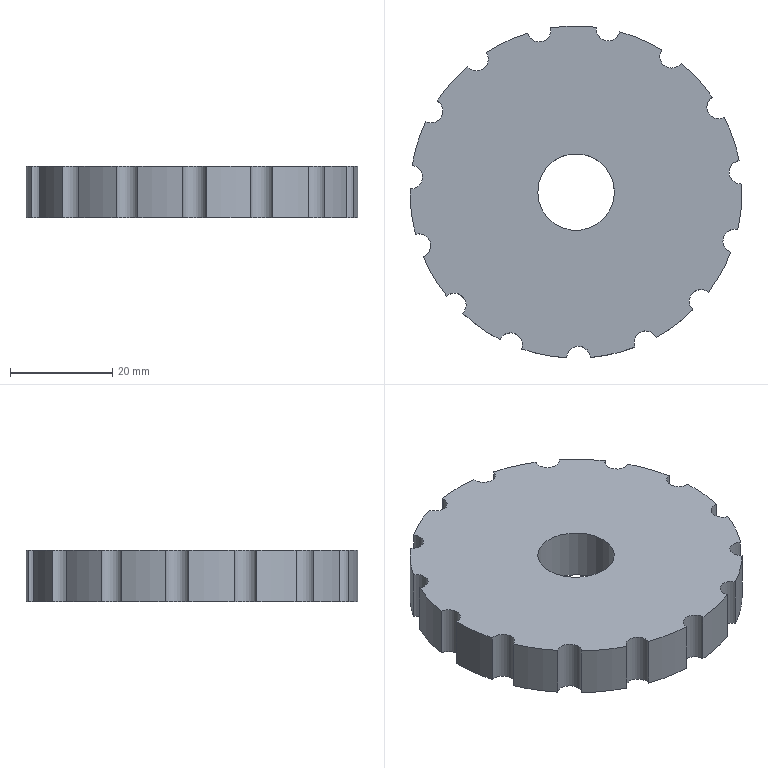Part | NX | features DATUM_CSYS 2, CYLINDER 1, EXTRUDE 1, SKETCH 1 | 1 solid | 33 faces | box 65 x 64.948 x 10 mm | volume 30179 mm3 | cylinder 31 | plane 2 | commonest cylinder face diameters 4.618 x15 65 x15 15 x1
STEP:
#1=CARTESIAN_POINT('',(16.782,27.832,0.));
#2=VERTEX_POINT('',#1);
#3=CARTESIAN_POINT('',(16.782,27.832,10.));
#4=VERTEX_POINT('',#3);
#5=CARTESIAN_POINT('',(16.782,27.832,0.));
#6=DIRECTION('',(0.,0.,1.));
#7=VECTOR('',#6,1000.);
#8=LINE('',#5,#7);
#9=EDGE_CURVE('',#2,#4,#8,.T.);
#10=ORIENTED_EDGE('',*,*,#9,.F.);
#11=CARTESIAN_POINT('',(8.539,31.358,0.));
#12=VERTEX_POINT('',#11);
#13=CARTESIAN_POINT('',(0.,0.,0.));
#14=DIRECTION('',(0.,0.,1.));
#15=DIRECTION('',(1.,0.,0.));
#16=AXIS2_PLACEMENT_3D('',#13,#14,#15);
#17=CIRCLE('',#16,32.5);
#18=EDGE_CURVE('',#2,#12,#17,.T.);
#19=ORIENTED_EDGE('',*,*,#18,.T.);
#20=CARTESIAN_POINT('',(8.539,31.358,10.));
#21=VERTEX_POINT('',#20);
#22=CARTESIAN_POINT('',(8.539,31.358,0.));
#23=DIRECTION('',(0.,0.,1.));
#24=VECTOR('',#23,1000.);
#25=LINE('',#22,#24);
#26=EDGE_CURVE('',#21,#12,#25,.F.);
#27=ORIENTED_EDGE('',*,*,#26,.F.);
#28=CARTESIAN_POINT('',(0.,0.,10.));
#29=DIRECTION('',(0.,0.,-1.));
#30=DIRECTION('',(1.,0.,0.));
#31=AXIS2_PLACEMENT_3D('',#28,#29,#30);
#32=CIRCLE('',#31,32.5);
#33=EDGE_CURVE('',#21,#4,#32,.T.);
#34=ORIENTED_EDGE('',*,*,#33,.T.);
#35=EDGE_LOOP('',(#10,#19,#27,#34));
#36=FACE_BOUND('',#35,.T.);
#37=CARTESIAN_POINT('',(0.,0.,0.));
#38=DIRECTION('',(0.,0.,1.));
#39=DIRECTION('',(1.,0.,0.));
#40=AXIS2_PLACEMENT_3D('',#37,#38,#39);
#41=CYLINDRICAL_SURFACE('',#40,32.5);
#42=ADVANCED_FACE('',(#36),#41,.T.);
#43=CARTESIAN_POINT('',(25.925,-19.599,0.));
#44=VERTEX_POINT('',#43);
#45=CARTESIAN_POINT('',(25.925,-19.599,10.));
#46=VERTEX_POINT('',#45);
#47=CARTESIAN_POINT('',(25.925,-19.599,0.));
#48=DIRECTION('',(0.,0.,1.));
#49=VECTOR('',#48,1000.);
#50=LINE('',#47,#49);
#51=EDGE_CURVE('',#44,#46,#50,.T.);
#52=ORIENTED_EDGE('',*,*,#51,.F.);
#53=CARTESIAN_POINT('',(30.294,-11.77,0.));
#54=VERTEX_POINT('',#53);
#55=CARTESIAN_POINT('',(0.,0.,0.));
#56=DIRECTION('',(0.,0.,1.));
#57=DIRECTION('',(1.,0.,0.));
#58=AXIS2_PLACEMENT_3D('',#55,#56,#57);
#59=CIRCLE('',#58,32.5);
#60=EDGE_CURVE('',#44,#54,#59,.T.);
#61=ORIENTED_EDGE('',*,*,#60,.T.);
#62=CARTESIAN_POINT('',(30.294,-11.77,10.));
#63=VERTEX_POINT('',#62);
#64=CARTESIAN_POINT('',(30.294,-11.77,0.));
#65=DIRECTION('',(0.,0.,1.));
#66=VECTOR('',#65,1000.);
#67=LINE('',#64,#66);
#68=EDGE_CURVE('',#63,#54,#67,.F.);
#69=ORIENTED_EDGE('',*,*,#68,.F.);
#70=CARTESIAN_POINT('',(0.,0.,10.));
#71=DIRECTION('',(0.,0.,-1.));
#72=DIRECTION('',(1.,0.,0.));
#73=AXIS2_PLACEMENT_3D('',#70,#71,#72);
#74=CIRCLE('',#73,32.5);
#75=EDGE_CURVE('',#63,#46,#74,.T.);
#76=ORIENTED_EDGE('',*,*,#75,.T.);
#77=EDGE_LOOP('',(#52,#61,#69,#76));
#78=FACE_BOUND('',#77,.T.);
#79=CARTESIAN_POINT('',(0.,0.,0.));
#80=DIRECTION('',(0.,0.,1.));
#81=DIRECTION('',(1.,0.,0.));
#82=AXIS2_PLACEMENT_3D('',#79,#80,#81);
#83=CYLINDRICAL_SURFACE('',#82,32.5);
#84=ADVANCED_FACE('',(#78),#83,.T.);
#85=CARTESIAN_POINT('',(20.555,25.174,10.));
#86=VERTEX_POINT('',#85);
#87=CARTESIAN_POINT('',(20.555,25.174,0.));
#88=VERTEX_POINT('',#87);
#89=CARTESIAN_POINT('',(20.555,25.174,0.));
#90=DIRECTION('',(0.,0.,1.));
#91=VECTOR('',#90,1000.);
#92=LINE('',#89,#91);
#93=EDGE_CURVE('',#86,#88,#92,.F.);
#94=ORIENTED_EDGE('',*,*,#93,.F.);
#95=CARTESIAN_POINT('',(26.651,18.6,10.));
#96=VERTEX_POINT('',#95);
#97=CARTESIAN_POINT('',(0.,0.,10.));
#98=DIRECTION('',(0.,0.,-1.));
#99=DIRECTION('',(1.,0.,0.));
#100=AXIS2_PLACEMENT_3D('',#97,#98,#99);
#101=CIRCLE('',#100,32.5);
#102=EDGE_CURVE('',#86,#96,#101,.T.);
#103=ORIENTED_EDGE('',*,*,#102,.T.);
#104=CARTESIAN_POINT('',(26.651,18.6,0.));
#105=VERTEX_POINT('',#104);
#106=CARTESIAN_POINT('',(26.651,18.6,0.));
#107=DIRECTION('',(0.,0.,1.));
#108=VECTOR('',#107,1000.);
#109=LINE('',#106,#108);
#110=EDGE_CURVE('',#105,#96,#109,.T.);
#111=ORIENTED_EDGE('',*,*,#110,.F.);
#112=CARTESIAN_POINT('',(0.,0.,0.));
#113=DIRECTION('',(0.,0.,1.));
#114=DIRECTION('',(1.,0.,0.));
#115=AXIS2_PLACEMENT_3D('',#112,#113,#114);
#116=CIRCLE('',#115,32.5);
#117=EDGE_CURVE('',#105,#88,#116,.T.);
#118=ORIENTED_EDGE('',*,*,#117,.T.);
#119=EDGE_LOOP('',(#94,#103,#111,#118));
#120=FACE_BOUND('',#119,.T.);
#121=CARTESIAN_POINT('',(0.,0.,0.));
#122=DIRECTION('',(0.,0.,1.));
#123=DIRECTION('',(1.,0.,0.));
#124=AXIS2_PLACEMENT_3D('',#121,#122,#123);
#125=CYLINDRICAL_SURFACE('',#124,32.5);
#126=ADVANCED_FACE('',(#120),#125,.T.);
#127=CARTESIAN_POINT('',(31.656,-7.36,0.));
#128=VERTEX_POINT('',#127);
#129=CARTESIAN_POINT('',(31.656,-7.36,10.));
#130=VERTEX_POINT('',#129);
#131=CARTESIAN_POINT('',(31.656,-7.36,0.));
#132=DIRECTION('',(0.,0.,1.));
#133=VECTOR('',#132,1000.);
#134=LINE('',#131,#133);
#135=EDGE_CURVE('',#128,#130,#134,.T.);
#136=ORIENTED_EDGE('',*,*,#135,.F.);
#137=CARTESIAN_POINT('',(32.462,1.569,0.));
#138=VERTEX_POINT('',#137);
#139=CARTESIAN_POINT('',(0.,0.,0.));
#140=DIRECTION('',(0.,0.,1.));
#141=DIRECTION('',(1.,0.,0.));
#142=AXIS2_PLACEMENT_3D('',#139,#140,#141);
#143=CIRCLE('',#142,32.5);
#144=EDGE_CURVE('',#128,#138,#143,.T.);
#145=ORIENTED_EDGE('',*,*,#144,.T.);
#146=CARTESIAN_POINT('',(32.462,1.569,10.));
#147=VERTEX_POINT('',#146);
#148=CARTESIAN_POINT('',(32.462,1.569,0.));
#149=DIRECTION('',(0.,0.,1.));
#150=VECTOR('',#149,1000.);
#151=LINE('',#148,#150);
#152=EDGE_CURVE('',#147,#138,#151,.F.);
#153=ORIENTED_EDGE('',*,*,#152,.F.);
#154=CARTESIAN_POINT('',(0.,0.,10.));
#155=DIRECTION('',(0.,0.,-1.));
#156=DIRECTION('',(1.,0.,0.));
#157=AXIS2_PLACEMENT_3D('',#154,#155,#156);
#158=CIRCLE('',#157,32.5);
#159=EDGE_CURVE('',#147,#130,#158,.T.);
#160=ORIENTED_EDGE('',*,*,#159,.T.);
#161=EDGE_LOOP('',(#136,#145,#153,#160));
#162=FACE_BOUND('',#161,.T.);
#163=CARTESIAN_POINT('',(0.,0.,0.));
#164=DIRECTION('',(0.,0.,1.));
#165=DIRECTION('',(1.,0.,0.));
#166=AXIS2_PLACEMENT_3D('',#163,#164,#165);
#167=CYLINDRICAL_SURFACE('',#166,32.5);
#168=ADVANCED_FACE('',(#162),#167,.T.);
#169=CARTESIAN_POINT('',(2.782,-32.381,0.));
#170=VERTEX_POINT('',#169);
#171=CARTESIAN_POINT('',(2.782,-32.381,10.));
#172=VERTEX_POINT('',#171);
#173=CARTESIAN_POINT('',(2.782,-32.381,0.));
#174=DIRECTION('',(0.,0.,1.));
#175=VECTOR('',#174,1000.);
#176=LINE('',#173,#175);
#177=EDGE_CURVE('',#170,#172,#176,.T.);
#178=ORIENTED_EDGE('',*,*,#177,.F.);
#179=CARTESIAN_POINT('',(11.524,-30.388,0.));
#180=VERTEX_POINT('',#179);
#181=CARTESIAN_POINT('',(0.,0.,0.));
#182=DIRECTION('',(0.,0.,1.));
#183=DIRECTION('',(1.,0.,0.));
#184=AXIS2_PLACEMENT_3D('',#181,#182,#183);
#185=CIRCLE('',#184,32.5);
#186=EDGE_CURVE('',#170,#180,#185,.T.);
#187=ORIENTED_EDGE('',*,*,#186,.T.);
#188=CARTESIAN_POINT('',(11.524,-30.388,10.));
#189=VERTEX_POINT('',#188);
#190=CARTESIAN_POINT('',(11.524,-30.388,0.));
#191=DIRECTION('',(0.,0.,1.));
#192=VECTOR('',#191,1000.);
#193=LINE('',#190,#192);
#194=EDGE_CURVE('',#189,#180,#193,.F.);
#195=ORIENTED_EDGE('',*,*,#194,.F.);
#196=CARTESIAN_POINT('',(0.,0.,10.));
#197=DIRECTION('',(0.,0.,-1.));
#198=DIRECTION('',(1.,0.,0.));
#199=AXIS2_PLACEMENT_3D('',#196,#197,#198);
#200=CIRCLE('',#199,32.5);
#201=EDGE_CURVE('',#189,#172,#200,.T.);
#202=ORIENTED_EDGE('',*,*,#201,.T.);
#203=EDGE_LOOP('',(#178,#187,#195,#202));
#204=FACE_BOUND('',#203,.T.);
#205=CARTESIAN_POINT('',(0.,0.,0.));
#206=DIRECTION('',(0.,0.,1.));
#207=DIRECTION('',(1.,0.,0.));
#208=AXIS2_PLACEMENT_3D('',#205,#206,#207);
#209=CYLINDRICAL_SURFACE('',#208,32.5);
#210=ADVANCED_FACE('',(#204),#209,.T.);
#211=CARTESIAN_POINT('',(4.011,32.252,0.));
#212=VERTEX_POINT('',#211);
#213=CARTESIAN_POINT('',(4.011,32.252,10.));
#214=VERTEX_POINT('',#213);
#215=CARTESIAN_POINT('',(4.011,32.252,0.));
#216=DIRECTION('',(0.,0.,1.));
#217=VECTOR('',#216,1000.);
#218=LINE('',#215,#217);
#219=EDGE_CURVE('',#212,#214,#218,.T.);
#220=ORIENTED_EDGE('',*,*,#219,.F.);
#221=CARTESIAN_POINT('',(-4.954,32.12,0.));
#222=VERTEX_POINT('',#221);
#223=CARTESIAN_POINT('',(0.,0.,0.));
#224=DIRECTION('',(0.,0.,1.));
#225=DIRECTION('',(1.,0.,0.));
#226=AXIS2_PLACEMENT_3D('',#223,#224,#225);
#227=CIRCLE('',#226,32.5);
#228=EDGE_CURVE('',#212,#222,#227,.T.);
#229=ORIENTED_EDGE('',*,*,#228,.T.);
#230=CARTESIAN_POINT('',(-4.954,32.12,10.));
#231=VERTEX_POINT('',#230);
#232=CARTESIAN_POINT('',(-4.954,32.12,0.));
#233=DIRECTION('',(0.,0.,1.));
#234=VECTOR('',#233,1000.);
#235=LINE('',#232,#234);
#236=EDGE_CURVE('',#231,#222,#235,.F.);
#237=ORIENTED_EDGE('',*,*,#236,.F.);
#238=CARTESIAN_POINT('',(0.,0.,10.));
#239=DIRECTION('',(0.,0.,-1.));
#240=DIRECTION('',(1.,0.,0.));
#241=AXIS2_PLACEMENT_3D('',#238,#239,#240);
#242=CIRCLE('',#241,32.5);
#243=EDGE_CURVE('',#231,#214,#242,.T.);
#244=ORIENTED_EDGE('',*,*,#243,.T.);
#245=EDGE_LOOP('',(#220,#229,#237,#244));
#246=FACE_BOUND('',#245,.T.);
#247=CARTESIAN_POINT('',(0.,0.,0.));
#248=DIRECTION('',(0.,0.,1.));
#249=DIRECTION('',(1.,0.,0.));
#250=AXIS2_PLACEMENT_3D('',#247,#248,#249);
#251=CYLINDRICAL_SURFACE('',#250,32.5);
#252=ADVANCED_FACE('',(#246),#251,.T.);
#253=CARTESIAN_POINT('',(22.888,-23.074,10.));
#254=VERTEX_POINT('',#253);
#255=CARTESIAN_POINT('',(22.888,-23.074,0.));
#256=VERTEX_POINT('',#255);
#257=CARTESIAN_POINT('',(22.888,-23.074,0.));
#258=DIRECTION('',(0.,0.,1.));
#259=VECTOR('',#258,1000.);
#260=LINE('',#257,#259);
#261=EDGE_CURVE('',#254,#256,#260,.F.);
#262=ORIENTED_EDGE('',*,*,#261,.F.);
#263=CARTESIAN_POINT('',(15.712,-28.45,10.));
#264=VERTEX_POINT('',#263);
#265=CARTESIAN_POINT('',(0.,0.,10.));
#266=DIRECTION('',(0.,0.,-1.));
#267=DIRECTION('',(1.,0.,0.));
#268=AXIS2_PLACEMENT_3D('',#265,#266,#267);
#269=CIRCLE('',#268,32.5);
#270=EDGE_CURVE('',#254,#264,#269,.T.);
#271=ORIENTED_EDGE('',*,*,#270,.T.);
#272=CARTESIAN_POINT('',(15.712,-28.45,0.));
#273=VERTEX_POINT('',#272);
#274=CARTESIAN_POINT('',(15.712,-28.45,0.));
#275=DIRECTION('',(0.,0.,1.));
#276=VECTOR('',#275,1000.);
#277=LINE('',#274,#276);
#278=EDGE_CURVE('',#273,#264,#277,.T.);
#279=ORIENTED_EDGE('',*,*,#278,.F.);
#280=CARTESIAN_POINT('',(0.,0.,0.));
#281=DIRECTION('',(0.,0.,1.));
#282=DIRECTION('',(1.,0.,0.));
#283=AXIS2_PLACEMENT_3D('',#280,#281,#282);
#284=CIRCLE('',#283,32.5);
#285=EDGE_CURVE('',#273,#256,#284,.T.);
#286=ORIENTED_EDGE('',*,*,#285,.T.);
#287=EDGE_LOOP('',(#262,#271,#279,#286));
#288=FACE_BOUND('',#287,.T.);
#289=CARTESIAN_POINT('',(0.,0.,0.));
#290=DIRECTION('',(0.,0.,1.));
#291=DIRECTION('',(1.,0.,0.));
#292=AXIS2_PLACEMENT_3D('',#289,#290,#291);
#293=CYLINDRICAL_SURFACE('',#292,32.5);
#294=ADVANCED_FACE('',(#288),#293,.T.);
#295=CARTESIAN_POINT('',(-29.434,13.781,0.));
#296=VERTEX_POINT('',#295);
#297=CARTESIAN_POINT('',(-29.434,13.781,10.));
#298=VERTEX_POINT('',#297);
#299=CARTESIAN_POINT('',(-29.434,13.781,0.));
#300=DIRECTION('',(0.,0.,1.));
#301=VECTOR('',#300,1000.);
#302=LINE('',#299,#301);
#303=EDGE_CURVE('',#296,#298,#302,.T.);
#304=ORIENTED_EDGE('',*,*,#303,.F.);
#305=CARTESIAN_POINT('',(-32.079,5.214,0.));
#306=VERTEX_POINT('',#305);
#307=CARTESIAN_POINT('',(0.,0.,0.));
#308=DIRECTION('',(0.,0.,1.));
#309=DIRECTION('',(1.,0.,0.));
#310=AXIS2_PLACEMENT_3D('',#307,#308,#309);
#311=CIRCLE('',#310,32.5);
#312=EDGE_CURVE('',#296,#306,#311,.T.);
#313=ORIENTED_EDGE('',*,*,#312,.T.);
#314=CARTESIAN_POINT('',(-32.079,5.214,10.));
#315=VERTEX_POINT('',#314);
#316=CARTESIAN_POINT('',(-32.079,5.214,0.));
#317=DIRECTION('',(0.,0.,1.));
#318=VECTOR('',#317,1000.);
#319=LINE('',#316,#318);
#320=EDGE_CURVE('',#315,#306,#319,.F.);
#321=ORIENTED_EDGE('',*,*,#320,.F.);
#322=CARTESIAN_POINT('',(0.,0.,10.));
#323=DIRECTION('',(0.,0.,-1.));
#324=DIRECTION('',(1.,0.,0.));
#325=AXIS2_PLACEMENT_3D('',#322,#323,#324);
#326=CIRCLE('',#325,32.5);
#327=EDGE_CURVE('',#315,#298,#326,.T.);
#328=ORIENTED_EDGE('',*,*,#327,.T.);
#329=EDGE_LOOP('',(#304,#313,#321,#328));
#330=FACE_BOUND('',#329,.T.);
#331=CARTESIAN_POINT('',(0.,0.,0.));
#332=DIRECTION('',(0.,0.,1.));
#333=DIRECTION('',(1.,0.,0.));
#334=AXIS2_PLACEMENT_3D('',#331,#332,#333);
#335=CYLINDRICAL_SURFACE('',#334,32.5);
#336=ADVANCED_FACE('',(#330),#335,.T.);
#337=CARTESIAN_POINT('',(-29.936,-12.652,0.));
#338=VERTEX_POINT('',#337);
#339=CARTESIAN_POINT('',(-29.936,-12.652,10.));
#340=VERTEX_POINT('',#339);
#341=CARTESIAN_POINT('',(-29.936,-12.652,0.));
#342=DIRECTION('',(0.,0.,1.));
#343=VECTOR('',#342,1000.);
#344=LINE('',#341,#343);
#345=EDGE_CURVE('',#338,#340,#344,.T.);
#346=ORIENTED_EDGE('',*,*,#345,.F.);
#347=CARTESIAN_POINT('',(-25.34,-20.35,0.));
#348=VERTEX_POINT('',#347);
#349=CARTESIAN_POINT('',(0.,0.,0.));
#350=DIRECTION('',(0.,0.,1.));
#351=DIRECTION('',(1.,0.,0.));
#352=AXIS2_PLACEMENT_3D('',#349,#350,#351);
#353=CIRCLE('',#352,32.5);
#354=EDGE_CURVE('',#338,#348,#353,.T.);
#355=ORIENTED_EDGE('',*,*,#354,.T.);
#356=CARTESIAN_POINT('',(-25.34,-20.35,10.));
#357=VERTEX_POINT('',#356);
#358=CARTESIAN_POINT('',(-25.34,-20.35,0.));
#359=DIRECTION('',(0.,0.,1.));
#360=VECTOR('',#359,1000.);
#361=LINE('',#358,#360);
#362=EDGE_CURVE('',#357,#348,#361,.F.);
#363=ORIENTED_EDGE('',*,*,#362,.F.);
#364=CARTESIAN_POINT('',(0.,0.,10.));
#365=DIRECTION('',(0.,0.,-1.));
#366=DIRECTION('',(1.,0.,0.));
#367=AXIS2_PLACEMENT_3D('',#364,#365,#366);
#368=CIRCLE('',#367,32.5);
#369=EDGE_CURVE('',#357,#340,#368,.T.);
#370=ORIENTED_EDGE('',*,*,#369,.T.);
#371=EDGE_LOOP('',(#346,#355,#363,#370));
#372=FACE_BOUND('',#371,.T.);
#373=CARTESIAN_POINT('',(0.,0.,0.));
#374=DIRECTION('',(0.,0.,1.));
#375=DIRECTION('',(1.,0.,0.));
#376=AXIS2_PLACEMENT_3D('',#373,#374,#375);
#377=CYLINDRICAL_SURFACE('',#376,32.5);
#378=ADVANCED_FACE('',(#372),#377,.T.);
#379=CARTESIAN_POINT('',(-31.426,-8.284,10.));
#380=VERTEX_POINT('',#379);
#381=CARTESIAN_POINT('',(-31.426,-8.284,0.));
#382=VERTEX_POINT('',#381);
#383=CARTESIAN_POINT('',(-31.426,-8.284,0.));
#384=DIRECTION('',(0.,0.,1.));
#385=VECTOR('',#384,1000.);
#386=LINE('',#383,#385);
#387=EDGE_CURVE('',#380,#382,#386,.F.);
#388=ORIENTED_EDGE('',*,*,#387,.F.);
#389=CARTESIAN_POINT('',(-32.494,0.6177,10.));
#390=VERTEX_POINT('',#389);
#391=CARTESIAN_POINT('',(0.,0.,10.));
#392=DIRECTION('',(0.,0.,-1.));
#393=DIRECTION('',(1.,0.,0.));
#394=AXIS2_PLACEMENT_3D('',#391,#392,#393);
#395=CIRCLE('',#394,32.5);
#396=EDGE_CURVE('',#380,#390,#395,.T.);
#397=ORIENTED_EDGE('',*,*,#396,.T.);
#398=CARTESIAN_POINT('',(-32.494,0.6177,0.));
#399=VERTEX_POINT('',#398);
#400=CARTESIAN_POINT('',(-32.494,0.6177,0.));
#401=DIRECTION('',(0.,0.,1.));
#402=VECTOR('',#401,1000.);
#403=LINE('',#400,#402);
#404=EDGE_CURVE('',#399,#390,#403,.T.);
#405=ORIENTED_EDGE('',*,*,#404,.F.);
#406=CARTESIAN_POINT('',(0.,0.,0.));
#407=DIRECTION('',(0.,0.,1.));
#408=DIRECTION('',(1.,0.,0.));
#409=AXIS2_PLACEMENT_3D('',#406,#407,#408);
#410=CIRCLE('',#409,32.5);
#411=EDGE_CURVE('',#399,#382,#410,.T.);
#412=ORIENTED_EDGE('',*,*,#411,.T.);
#413=EDGE_LOOP('',(#388,#397,#405,#412));
#414=FACE_BOUND('',#413,.T.);
#415=CARTESIAN_POINT('',(0.,0.,0.));
#416=DIRECTION('',(0.,0.,1.));
#417=DIRECTION('',(1.,0.,0.));
#418=AXIS2_PLACEMENT_3D('',#415,#416,#417);
#419=CYLINDRICAL_SURFACE('',#418,32.5);
#420=ADVANCED_FACE('',(#414),#419,.T.);
#421=CARTESIAN_POINT('',(-22.202,-23.734,0.));
#422=VERTEX_POINT('',#421);
#423=CARTESIAN_POINT('',(-22.202,-23.734,10.));
#424=VERTEX_POINT('',#423);
#425=CARTESIAN_POINT('',(-22.202,-23.734,0.));
#426=DIRECTION('',(0.,0.,1.));
#427=VECTOR('',#426,1000.);
#428=LINE('',#425,#427);
#429=EDGE_CURVE('',#422,#424,#428,.T.);
#430=ORIENTED_EDGE('',*,*,#429,.F.);
#431=CARTESIAN_POINT('',(-14.872,-28.898,0.));
#432=VERTEX_POINT('',#431);
#433=CARTESIAN_POINT('',(0.,0.,0.));
#434=DIRECTION('',(0.,0.,1.));
#435=DIRECTION('',(1.,0.,0.));
#436=AXIS2_PLACEMENT_3D('',#433,#434,#435);
#437=CIRCLE('',#436,32.5);
#438=EDGE_CURVE('',#422,#432,#437,.T.);
#439=ORIENTED_EDGE('',*,*,#438,.T.);
#440=CARTESIAN_POINT('',(-14.872,-28.898,10.));
#441=VERTEX_POINT('',#440);
#442=CARTESIAN_POINT('',(-14.872,-28.898,0.));
#443=DIRECTION('',(0.,0.,1.));
#444=VECTOR('',#443,1000.);
#445=LINE('',#442,#444);
#446=EDGE_CURVE('',#441,#432,#445,.F.);
#447=ORIENTED_EDGE('',*,*,#446,.F.);
#448=CARTESIAN_POINT('',(0.,0.,10.));
#449=DIRECTION('',(0.,0.,-1.));
#450=DIRECTION('',(1.,0.,0.));
#451=AXIS2_PLACEMENT_3D('',#448,#449,#450);
#452=CIRCLE('',#451,32.5);
#453=EDGE_CURVE('',#441,#424,#452,.T.);
#454=ORIENTED_EDGE('',*,*,#453,.T.);
#455=EDGE_LOOP('',(#430,#439,#447,#454));
#456=FACE_BOUND('',#455,.T.);
#457=CARTESIAN_POINT('',(0.,0.,0.));
#458=DIRECTION('',(0.,0.,1.));
#459=DIRECTION('',(1.,0.,0.));
#460=AXIS2_PLACEMENT_3D('',#457,#458,#459);
#461=CYLINDRICAL_SURFACE('',#460,32.5);
#462=ADVANCED_FACE('',(#456),#461,.T.);
#463=CARTESIAN_POINT('',(-27.185,17.811,10.));
#464=VERTEX_POINT('',#463);
#465=CARTESIAN_POINT('',(-27.185,17.811,0.));
#466=VERTEX_POINT('',#465);
#467=CARTESIAN_POINT('',(-27.185,17.811,0.));
#468=DIRECTION('',(0.,0.,1.));
#469=VECTOR('',#468,1000.);
#470=LINE('',#467,#469);
#471=EDGE_CURVE('',#464,#466,#470,.F.);
#472=ORIENTED_EDGE('',*,*,#471,.F.);
#473=CARTESIAN_POINT('',(-21.284,24.561,10.));
#474=VERTEX_POINT('',#473);
#475=CARTESIAN_POINT('',(0.,0.,10.));
#476=DIRECTION('',(0.,0.,-1.));
#477=DIRECTION('',(1.,0.,0.));
#478=AXIS2_PLACEMENT_3D('',#475,#476,#477);
#479=CIRCLE('',#478,32.5);
#480=EDGE_CURVE('',#464,#474,#479,.T.);
#481=ORIENTED_EDGE('',*,*,#480,.T.);
#482=CARTESIAN_POINT('',(-21.284,24.561,0.));
#483=VERTEX_POINT('',#482);
#484=CARTESIAN_POINT('',(-21.284,24.561,0.));
#485=DIRECTION('',(0.,0.,1.));
#486=VECTOR('',#485,1000.);
#487=LINE('',#484,#486);
#488=EDGE_CURVE('',#483,#474,#487,.T.);
#489=ORIENTED_EDGE('',*,*,#488,.F.);
#490=CARTESIAN_POINT('',(0.,0.,0.));
#491=DIRECTION('',(0.,0.,1.));
#492=DIRECTION('',(1.,0.,0.));
#493=AXIS2_PLACEMENT_3D('',#490,#491,#492);
#494=CIRCLE('',#493,32.5);
#495=EDGE_CURVE('',#483,#466,#494,.T.);
#496=ORIENTED_EDGE('',*,*,#495,.T.);
#497=EDGE_LOOP('',(#472,#481,#489,#496));
#498=FACE_BOUND('',#497,.T.);
#499=CARTESIAN_POINT('',(0.,0.,0.));
#500=DIRECTION('',(0.,0.,1.));
#501=DIRECTION('',(1.,0.,0.));
#502=AXIS2_PLACEMENT_3D('',#499,#500,#501);
#503=CYLINDRICAL_SURFACE('',#502,32.5);
#504=ADVANCED_FACE('',(#498),#503,.T.);
#505=CARTESIAN_POINT('',(-1.833,-32.448,10.));
#506=VERTEX_POINT('',#505);
#507=CARTESIAN_POINT('',(-1.833,-32.448,0.));
#508=VERTEX_POINT('',#507);
#509=CARTESIAN_POINT('',(-1.833,-32.448,0.));
#510=DIRECTION('',(0.,0.,1.));
#511=VECTOR('',#510,1000.);
#512=LINE('',#509,#511);
#513=EDGE_CURVE('',#506,#508,#512,.F.);
#514=ORIENTED_EDGE('',*,*,#513,.F.);
#515=CARTESIAN_POINT('',(-10.629,-30.713,10.));
#516=VERTEX_POINT('',#515);
#517=CARTESIAN_POINT('',(0.,0.,10.));
#518=DIRECTION('',(0.,0.,-1.));
#519=DIRECTION('',(1.,0.,0.));
#520=AXIS2_PLACEMENT_3D('',#517,#518,#519);
#521=CIRCLE('',#520,32.5);
#522=EDGE_CURVE('',#506,#516,#521,.T.);
#523=ORIENTED_EDGE('',*,*,#522,.T.);
#524=CARTESIAN_POINT('',(-10.629,-30.713,0.));
#525=VERTEX_POINT('',#524);
#526=CARTESIAN_POINT('',(-10.629,-30.713,0.));
#527=DIRECTION('',(0.,0.,1.));
#528=VECTOR('',#527,1000.);
#529=LINE('',#526,#528);
#530=EDGE_CURVE('',#525,#516,#529,.T.);
#531=ORIENTED_EDGE('',*,*,#530,.F.);
#532=CARTESIAN_POINT('',(0.,0.,0.));
#533=DIRECTION('',(0.,0.,1.));
#534=DIRECTION('',(1.,0.,0.));
#535=AXIS2_PLACEMENT_3D('',#532,#533,#534);
#536=CIRCLE('',#535,32.5);
#537=EDGE_CURVE('',#525,#508,#536,.T.);
#538=ORIENTED_EDGE('',*,*,#537,.T.);
#539=EDGE_LOOP('',(#514,#523,#531,#538));
#540=FACE_BOUND('',#539,.T.);
#541=CARTESIAN_POINT('',(0.,0.,0.));
#542=DIRECTION('',(0.,0.,1.));
#543=DIRECTION('',(1.,0.,0.));
#544=AXIS2_PLACEMENT_3D('',#541,#542,#543);
#545=CYLINDRICAL_SURFACE('',#544,32.5);
#546=ADVANCED_FACE('',(#540),#545,.T.);
#547=CARTESIAN_POINT('',(-17.59,27.328,10.));
#548=VERTEX_POINT('',#547);
#549=CARTESIAN_POINT('',(-17.59,27.328,0.));
#550=VERTEX_POINT('',#549);
#551=CARTESIAN_POINT('',(-17.59,27.328,0.));
#552=DIRECTION('',(0.,0.,1.));
#553=VECTOR('',#552,1000.);
#554=LINE('',#551,#553);
#555=EDGE_CURVE('',#548,#550,#554,.F.);
#556=ORIENTED_EDGE('',*,*,#555,.F.);
#557=CARTESIAN_POINT('',(-9.454,31.095,10.));
#558=VERTEX_POINT('',#557);
#559=CARTESIAN_POINT('',(0.,0.,10.));
#560=DIRECTION('',(0.,0.,-1.));
#561=DIRECTION('',(1.,0.,0.));
#562=AXIS2_PLACEMENT_3D('',#559,#560,#561);
#563=CIRCLE('',#562,32.5);
#564=EDGE_CURVE('',#548,#558,#563,.T.);
#565=ORIENTED_EDGE('',*,*,#564,.T.);
#566=CARTESIAN_POINT('',(-9.454,31.095,0.));
#567=VERTEX_POINT('',#566);
#568=CARTESIAN_POINT('',(-9.454,31.095,0.));
#569=DIRECTION('',(0.,0.,1.));
#570=VECTOR('',#569,1000.);
#571=LINE('',#568,#570);
#572=EDGE_CURVE('',#567,#558,#571,.T.);
#573=ORIENTED_EDGE('',*,*,#572,.F.);
#574=CARTESIAN_POINT('',(0.,0.,0.));
#575=DIRECTION('',(0.,0.,1.));
#576=DIRECTION('',(1.,0.,0.));
#577=AXIS2_PLACEMENT_3D('',#574,#575,#576);
#578=CIRCLE('',#577,32.5);
#579=EDGE_CURVE('',#567,#550,#578,.T.);
#580=ORIENTED_EDGE('',*,*,#579,.T.);
#581=EDGE_LOOP('',(#556,#565,#573,#580));
#582=FACE_BOUND('',#581,.T.);
#583=CARTESIAN_POINT('',(0.,0.,0.));
#584=DIRECTION('',(0.,0.,1.));
#585=DIRECTION('',(1.,0.,0.));
#586=AXIS2_PLACEMENT_3D('',#583,#584,#585);
#587=CYLINDRICAL_SURFACE('',#586,32.5);
#588=ADVANCED_FACE('',(#582),#587,.T.);
#589=CARTESIAN_POINT('',(18.716,26.57,10.));
#590=DIRECTION('',(0.,0.,1.));
#591=DIRECTION('',(-0.9781,0.2079,0.));
#592=AXIS2_PLACEMENT_3D('',#589,#590,#591);
#593=CIRCLE('',#592,2.309);
#594=EDGE_CURVE('',#4,#86,#593,.T.);
#595=ORIENTED_EDGE('',*,*,#594,.F.);
#596=ORIENTED_EDGE('',*,*,#33,.F.);
#597=CARTESIAN_POINT('',(6.291,31.885,10.));
#598=DIRECTION('',(0.,0.,1.));
#599=DIRECTION('',(-0.9781,-0.2079,0.));
#600=AXIS2_PLACEMENT_3D('',#597,#598,#599);
#601=CIRCLE('',#600,2.309);
#602=EDGE_CURVE('',#214,#21,#601,.T.);
#603=ORIENTED_EDGE('',*,*,#602,.F.);
#604=ORIENTED_EDGE('',*,*,#243,.F.);
#605=CARTESIAN_POINT('',(-7.222,31.687,10.));
#606=DIRECTION('',(0.,0.,1.));
#607=DIRECTION('',(-0.809,-0.5878,0.));
#608=AXIS2_PLACEMENT_3D('',#605,#606,#607);
#609=CIRCLE('',#608,2.309);
#610=EDGE_CURVE('',#558,#231,#609,.T.);
#611=ORIENTED_EDGE('',*,*,#610,.F.);
#612=ORIENTED_EDGE('',*,*,#564,.F.);
#613=CARTESIAN_POINT('',(-19.486,26.01,10.));
#614=DIRECTION('',(0.,0.,1.));
#615=DIRECTION('',(-0.5,-0.866,0.));
#616=AXIS2_PLACEMENT_3D('',#613,#614,#615);
#617=CIRCLE('',#616,2.309);
#618=EDGE_CURVE('',#474,#548,#617,.T.);
#619=ORIENTED_EDGE('',*,*,#618,.F.);
#620=ORIENTED_EDGE('',*,*,#480,.F.);
#621=CARTESIAN_POINT('',(-28.381,15.836,10.));
#622=DIRECTION('',(0.,0.,1.));
#623=DIRECTION('',(-0.1045,-0.9945,0.));
#624=AXIS2_PLACEMENT_3D('',#621,#622,#623);
#625=CIRCLE('',#624,2.309);
#626=EDGE_CURVE('',#298,#464,#625,.T.);
#627=ORIENTED_EDGE('',*,*,#626,.F.);
#628=ORIENTED_EDGE('',*,*,#327,.F.);
#629=CARTESIAN_POINT('',(-32.368,2.923,10.));
#630=DIRECTION('',(0.,0.,1.));
#631=DIRECTION('',(0.309,-0.9511,0.));
#632=AXIS2_PLACEMENT_3D('',#629,#630,#631);
#633=CIRCLE('',#632,2.309);
#634=EDGE_CURVE('',#390,#315,#633,.T.);
#635=ORIENTED_EDGE('',*,*,#634,.F.);
#636=ORIENTED_EDGE('',*,*,#396,.F.);
#637=CARTESIAN_POINT('',(-30.759,-10.495,10.));
#638=DIRECTION('',(0.,0.,1.));
#639=DIRECTION('',(0.6691,-0.7431,0.));
#640=AXIS2_PLACEMENT_3D('',#637,#638,#639);
#641=CIRCLE('',#640,2.309);
#642=EDGE_CURVE('',#340,#380,#641,.T.);
#643=ORIENTED_EDGE('',*,*,#642,.F.);
#644=ORIENTED_EDGE('',*,*,#369,.F.);
#645=CARTESIAN_POINT('',(-23.831,-22.098,10.));
#646=DIRECTION('',(0.,0.,1.));
#647=DIRECTION('',(0.9135,-0.4067,0.));
#648=AXIS2_PLACEMENT_3D('',#645,#646,#647);
#649=CIRCLE('',#648,2.309);
#650=EDGE_CURVE('',#424,#357,#649,.T.);
#651=ORIENTED_EDGE('',*,*,#650,.F.);
#652=ORIENTED_EDGE('',*,*,#453,.F.);
#653=CARTESIAN_POINT('',(-12.783,-29.881,10.));
#654=DIRECTION('',(0.,0.,1.));
#655=DIRECTION('',(1.,0.,0.));
#656=AXIS2_PLACEMENT_3D('',#653,#654,#655);
#657=CIRCLE('',#656,2.309);
#658=EDGE_CURVE('',#516,#441,#657,.T.);
#659=ORIENTED_EDGE('',*,*,#658,.F.);
#660=ORIENTED_EDGE('',*,*,#522,.F.);
#661=CARTESIAN_POINT('',(0.4761,-32.497,10.));
#662=DIRECTION('',(0.,0.,1.));
#663=DIRECTION('',(0.9135,0.4067,0.));
#664=AXIS2_PLACEMENT_3D('',#661,#662,#663);
#665=CIRCLE('',#664,2.309);
#666=EDGE_CURVE('',#172,#506,#665,.T.);
#667=ORIENTED_EDGE('',*,*,#666,.F.);
#668=ORIENTED_EDGE('',*,*,#201,.F.);
#669=CARTESIAN_POINT('',(13.652,-29.493,10.));
#670=DIRECTION('',(0.,0.,1.));
#671=DIRECTION('',(0.6691,0.7431,0.));
#672=AXIS2_PLACEMENT_3D('',#669,#670,#671);
#673=CIRCLE('',#672,2.309);
#674=EDGE_CURVE('',#264,#189,#673,.T.);
#675=ORIENTED_EDGE('',*,*,#674,.F.);
#676=ORIENTED_EDGE('',*,*,#270,.F.);
#677=CARTESIAN_POINT('',(24.468,-21.391,10.));
#678=DIRECTION('',(0.,0.,1.));
#679=DIRECTION('',(0.309,0.9511,0.));
#680=AXIS2_PLACEMENT_3D('',#677,#678,#679);
#681=CIRCLE('',#680,2.309);
#682=EDGE_CURVE('',#46,#254,#681,.T.);
#683=ORIENTED_EDGE('',*,*,#682,.F.);
#684=ORIENTED_EDGE('',*,*,#75,.F.);
#685=CARTESIAN_POINT('',(31.053,-9.589,10.));
#686=DIRECTION('',(0.,0.,1.));
#687=DIRECTION('',(-0.1045,0.9945,0.));
#688=AXIS2_PLACEMENT_3D('',#685,#686,#687);
#689=CIRCLE('',#688,2.309);
#690=EDGE_CURVE('',#130,#63,#689,.T.);
#691=ORIENTED_EDGE('',*,*,#690,.F.);
#692=ORIENTED_EDGE('',*,*,#159,.F.);
#693=CARTESIAN_POINT('',(31.912,6.152,10.));
#694=VERTEX_POINT('',#693);
#695=CARTESIAN_POINT('',(32.269,3.87,10.));
#696=DIRECTION('',(0.,0.,1.));
#697=DIRECTION('',(-0.5,0.866,0.));
#698=AXIS2_PLACEMENT_3D('',#695,#696,#697);
#699=CIRCLE('',#698,2.309);
#700=EDGE_CURVE('',#694,#147,#699,.T.);
#701=ORIENTED_EDGE('',*,*,#700,.F.);
#702=CARTESIAN_POINT('',(29.017,14.637,10.));
#703=VERTEX_POINT('',#702);
#704=CARTESIAN_POINT('',(0.,0.,10.));
#705=DIRECTION('',(0.,0.,-1.));
#706=DIRECTION('',(1.,0.,0.));
#707=AXIS2_PLACEMENT_3D('',#704,#705,#706);
#708=CIRCLE('',#707,32.5);
#709=EDGE_CURVE('',#703,#694,#708,.T.);
#710=ORIENTED_EDGE('',*,*,#709,.F.);
#711=CARTESIAN_POINT('',(27.905,16.661,10.));
#712=DIRECTION('',(0.,0.,1.));
#713=DIRECTION('',(-0.809,0.5878,0.));
#714=AXIS2_PLACEMENT_3D('',#711,#712,#713);
#715=CIRCLE('',#714,2.309);
#716=EDGE_CURVE('',#96,#703,#715,.T.);
#717=ORIENTED_EDGE('',*,*,#716,.F.);
#718=ORIENTED_EDGE('',*,*,#102,.F.);
#719=EDGE_LOOP('',(#595,#596,#603,#604,#611,#612,#619,#620,#627,#628,#635,#636,#643,#644,#651,#652,#659,#660,#667,#668,#675,#676,#683,#684,#691,#692,#701,#710,#717,#718));
#720=FACE_BOUND('',#719,.T.);
#721=CARTESIAN_POINT('',(7.5,0.,10.));
#722=VERTEX_POINT('',#721);
#723=CARTESIAN_POINT('',(0.,0.,10.));
#724=DIRECTION('',(0.,0.,1.));
#725=DIRECTION('',(1.,0.,0.));
#726=AXIS2_PLACEMENT_3D('',#723,#724,#725);
#727=CIRCLE('',#726,7.5);
#728=EDGE_CURVE('',#722,#722,#727,.T.);
#729=ORIENTED_EDGE('',*,*,#728,.F.);
#730=EDGE_LOOP('',(#729));
#731=FACE_BOUND('',#730,.T.);
#732=CARTESIAN_POINT('',(0.,0.,10.));
#733=DIRECTION('',(0.,0.,1.));
#734=DIRECTION('',(1.,0.,0.));
#735=AXIS2_PLACEMENT_3D('',#732,#733,#734);
#736=PLANE('',#735);
#737=ADVANCED_FACE('',(#720,#731),#736,.T.);
#738=CARTESIAN_POINT('',(18.716,26.57,0.));
#739=DIRECTION('',(0.,0.,-1.));
#740=DIRECTION('',(-1.,0.,0.));
#741=AXIS2_PLACEMENT_3D('',#738,#739,#740);
#742=CIRCLE('',#741,2.309);
#743=EDGE_CURVE('',#88,#2,#742,.T.);
#744=ORIENTED_EDGE('',*,*,#743,.F.);
#745=ORIENTED_EDGE('',*,*,#117,.F.);
#746=CARTESIAN_POINT('',(29.017,14.637,0.));
#747=VERTEX_POINT('',#746);
#748=CARTESIAN_POINT('',(27.905,16.661,0.));
#749=DIRECTION('',(0.,0.,-1.));
#750=DIRECTION('',(-1.,0.,0.));
#751=AXIS2_PLACEMENT_3D('',#748,#749,#750);
#752=CIRCLE('',#751,2.309);
#753=EDGE_CURVE('',#747,#105,#752,.T.);
#754=ORIENTED_EDGE('',*,*,#753,.F.);
#755=CARTESIAN_POINT('',(31.912,6.152,0.));
#756=VERTEX_POINT('',#755);
#757=CARTESIAN_POINT('',(0.,0.,0.));
#758=DIRECTION('',(0.,0.,1.));
#759=DIRECTION('',(1.,0.,0.));
#760=AXIS2_PLACEMENT_3D('',#757,#758,#759);
#761=CIRCLE('',#760,32.5);
#762=EDGE_CURVE('',#756,#747,#761,.T.);
#763=ORIENTED_EDGE('',*,*,#762,.F.);
#764=CARTESIAN_POINT('',(32.269,3.87,0.));
#765=DIRECTION('',(0.,0.,-1.));
#766=DIRECTION('',(-1.,0.,0.));
#767=AXIS2_PLACEMENT_3D('',#764,#765,#766);
#768=CIRCLE('',#767,2.309);
#769=EDGE_CURVE('',#138,#756,#768,.T.);
#770=ORIENTED_EDGE('',*,*,#769,.F.);
#771=ORIENTED_EDGE('',*,*,#144,.F.);
#772=CARTESIAN_POINT('',(31.053,-9.589,0.));
#773=DIRECTION('',(0.,0.,-1.));
#774=DIRECTION('',(-1.,0.,0.));
#775=AXIS2_PLACEMENT_3D('',#772,#773,#774);
#776=CIRCLE('',#775,2.309);
#777=EDGE_CURVE('',#54,#128,#776,.T.);
#778=ORIENTED_EDGE('',*,*,#777,.F.);
#779=ORIENTED_EDGE('',*,*,#60,.F.);
#780=CARTESIAN_POINT('',(24.468,-21.391,0.));
#781=DIRECTION('',(0.,0.,-1.));
#782=DIRECTION('',(-1.,0.,0.));
#783=AXIS2_PLACEMENT_3D('',#780,#781,#782);
#784=CIRCLE('',#783,2.309);
#785=EDGE_CURVE('',#256,#44,#784,.T.);
#786=ORIENTED_EDGE('',*,*,#785,.F.);
#787=ORIENTED_EDGE('',*,*,#285,.F.);
#788=CARTESIAN_POINT('',(13.652,-29.493,0.));
#789=DIRECTION('',(0.,0.,-1.));
#790=DIRECTION('',(-1.,0.,0.));
#791=AXIS2_PLACEMENT_3D('',#788,#789,#790);
#792=CIRCLE('',#791,2.309);
#793=EDGE_CURVE('',#180,#273,#792,.T.);
#794=ORIENTED_EDGE('',*,*,#793,.F.);
#795=ORIENTED_EDGE('',*,*,#186,.F.);
#796=CARTESIAN_POINT('',(0.4761,-32.497,0.));
#797=DIRECTION('',(0.,0.,-1.));
#798=DIRECTION('',(-1.,0.,0.));
#799=AXIS2_PLACEMENT_3D('',#796,#797,#798);
#800=CIRCLE('',#799,2.309);
#801=EDGE_CURVE('',#508,#170,#800,.T.);
#802=ORIENTED_EDGE('',*,*,#801,.F.);
#803=ORIENTED_EDGE('',*,*,#537,.F.);
#804=CARTESIAN_POINT('',(-12.783,-29.881,0.));
#805=DIRECTION('',(0.,0.,-1.));
#806=DIRECTION('',(-1.,0.,0.));
#807=AXIS2_PLACEMENT_3D('',#804,#805,#806);
#808=CIRCLE('',#807,2.309);
#809=EDGE_CURVE('',#432,#525,#808,.T.);
#810=ORIENTED_EDGE('',*,*,#809,.F.);
#811=ORIENTED_EDGE('',*,*,#438,.F.);
#812=CARTESIAN_POINT('',(-23.831,-22.098,0.));
#813=DIRECTION('',(0.,0.,-1.));
#814=DIRECTION('',(-1.,0.,0.));
#815=AXIS2_PLACEMENT_3D('',#812,#813,#814);
#816=CIRCLE('',#815,2.309);
#817=EDGE_CURVE('',#348,#422,#816,.T.);
#818=ORIENTED_EDGE('',*,*,#817,.F.);
#819=ORIENTED_EDGE('',*,*,#354,.F.);
#820=CARTESIAN_POINT('',(-30.759,-10.495,0.));
#821=DIRECTION('',(0.,0.,-1.));
#822=DIRECTION('',(-1.,0.,0.));
#823=AXIS2_PLACEMENT_3D('',#820,#821,#822);
#824=CIRCLE('',#823,2.309);
#825=EDGE_CURVE('',#382,#338,#824,.T.);
#826=ORIENTED_EDGE('',*,*,#825,.F.);
#827=ORIENTED_EDGE('',*,*,#411,.F.);
#828=CARTESIAN_POINT('',(-32.368,2.923,0.));
#829=DIRECTION('',(0.,0.,-1.));
#830=DIRECTION('',(-1.,0.,0.));
#831=AXIS2_PLACEMENT_3D('',#828,#829,#830);
#832=CIRCLE('',#831,2.309);
#833=EDGE_CURVE('',#306,#399,#832,.T.);
#834=ORIENTED_EDGE('',*,*,#833,.F.);
#835=ORIENTED_EDGE('',*,*,#312,.F.);
#836=CARTESIAN_POINT('',(-28.381,15.836,0.));
#837=DIRECTION('',(0.,0.,-1.));
#838=DIRECTION('',(-1.,0.,0.));
#839=AXIS2_PLACEMENT_3D('',#836,#837,#838);
#840=CIRCLE('',#839,2.309);
#841=EDGE_CURVE('',#466,#296,#840,.T.);
#842=ORIENTED_EDGE('',*,*,#841,.F.);
#843=ORIENTED_EDGE('',*,*,#495,.F.);
#844=CARTESIAN_POINT('',(-19.486,26.01,0.));
#845=DIRECTION('',(0.,0.,-1.));
#846=DIRECTION('',(-1.,0.,0.));
#847=AXIS2_PLACEMENT_3D('',#844,#845,#846);
#848=CIRCLE('',#847,2.309);
#849=EDGE_CURVE('',#550,#483,#848,.T.);
#850=ORIENTED_EDGE('',*,*,#849,.F.);
#851=ORIENTED_EDGE('',*,*,#579,.F.);
#852=CARTESIAN_POINT('',(-7.222,31.687,0.));
#853=DIRECTION('',(0.,0.,-1.));
#854=DIRECTION('',(-1.,0.,0.));
#855=AXIS2_PLACEMENT_3D('',#852,#853,#854);
#856=CIRCLE('',#855,2.309);
#857=EDGE_CURVE('',#222,#567,#856,.T.);
#858=ORIENTED_EDGE('',*,*,#857,.F.);
#859=ORIENTED_EDGE('',*,*,#228,.F.);
#860=CARTESIAN_POINT('',(6.291,31.885,0.));
#861=DIRECTION('',(0.,0.,-1.));
#862=DIRECTION('',(-1.,0.,0.));
#863=AXIS2_PLACEMENT_3D('',#860,#861,#862);
#864=CIRCLE('',#863,2.309);
#865=EDGE_CURVE('',#12,#212,#864,.T.);
#866=ORIENTED_EDGE('',*,*,#865,.F.);
#867=ORIENTED_EDGE('',*,*,#18,.F.);
#868=EDGE_LOOP('',(#744,#745,#754,#763,#770,#771,#778,#779,#786,#787,#794,#795,#802,#803,#810,#811,#818,#819,#826,#827,#834,#835,#842,#843,#850,#851,#858,#859,#866,#867));
#869=FACE_BOUND('',#868,.T.);
#870=CARTESIAN_POINT('',(-7.5,0.,0.));
#871=VERTEX_POINT('',#870);
#872=CARTESIAN_POINT('',(0.,0.,0.));
#873=DIRECTION('',(0.,0.,-1.));
#874=DIRECTION('',(-1.,0.,0.));
#875=AXIS2_PLACEMENT_3D('',#872,#873,#874);
#876=CIRCLE('',#875,7.5);
#877=EDGE_CURVE('',#871,#871,#876,.T.);
#878=ORIENTED_EDGE('',*,*,#877,.F.);
#879=EDGE_LOOP('',(#878));
#880=FACE_BOUND('',#879,.T.);
#881=CARTESIAN_POINT('',(0.,0.,0.));
#882=DIRECTION('',(0.,0.,-1.));
#883=DIRECTION('',(-1.,0.,0.));
#884=AXIS2_PLACEMENT_3D('',#881,#882,#883);
#885=PLANE('',#884);
#886=ADVANCED_FACE('',(#869,#880),#885,.T.);
#887=CARTESIAN_POINT('',(29.017,14.637,0.));
#888=DIRECTION('',(0.,0.,1.));
#889=VECTOR('',#888,1000.);
#890=LINE('',#887,#889);
#891=EDGE_CURVE('',#703,#747,#890,.F.);
#892=ORIENTED_EDGE('',*,*,#891,.F.);
#893=ORIENTED_EDGE('',*,*,#709,.T.);
#894=CARTESIAN_POINT('',(31.912,6.152,0.));
#895=DIRECTION('',(0.,0.,1.));
#896=VECTOR('',#895,1000.);
#897=LINE('',#894,#896);
#898=EDGE_CURVE('',#756,#694,#897,.T.);
#899=ORIENTED_EDGE('',*,*,#898,.F.);
#900=ORIENTED_EDGE('',*,*,#762,.T.);
#901=EDGE_LOOP('',(#892,#893,#899,#900));
#902=FACE_BOUND('',#901,.T.);
#903=CARTESIAN_POINT('',(0.,0.,0.));
#904=DIRECTION('',(0.,0.,1.));
#905=DIRECTION('',(1.,0.,0.));
#906=AXIS2_PLACEMENT_3D('',#903,#904,#905);
#907=CYLINDRICAL_SURFACE('',#906,32.5);
#908=ADVANCED_FACE('',(#902),#907,.T.);
#909=ORIENTED_EDGE('',*,*,#898,.T.);
#910=ORIENTED_EDGE('',*,*,#700,.T.);
#911=ORIENTED_EDGE('',*,*,#152,.T.);
#912=ORIENTED_EDGE('',*,*,#769,.T.);
#913=EDGE_LOOP('',(#909,#910,#911,#912));
#914=FACE_BOUND('',#913,.T.);
#915=CARTESIAN_POINT('',(32.269,3.87,-10.));
#916=DIRECTION('',(0.,0.,1.));
#917=DIRECTION('',(1.,0.,0.));
#918=AXIS2_PLACEMENT_3D('',#915,#916,#917);
#919=CYLINDRICAL_SURFACE('',#918,2.309);
#920=ADVANCED_FACE('',(#914),#919,.F.);
#921=ORIENTED_EDGE('',*,*,#572,.T.);
#922=ORIENTED_EDGE('',*,*,#610,.T.);
#923=ORIENTED_EDGE('',*,*,#236,.T.);
#924=ORIENTED_EDGE('',*,*,#857,.T.);
#925=EDGE_LOOP('',(#921,#922,#923,#924));
#926=FACE_BOUND('',#925,.T.);
#927=CARTESIAN_POINT('',(-7.222,31.687,-10.));
#928=DIRECTION('',(0.,0.,1.));
#929=DIRECTION('',(1.,0.,0.));
#930=AXIS2_PLACEMENT_3D('',#927,#928,#929);
#931=CYLINDRICAL_SURFACE('',#930,2.309);
#932=ADVANCED_FACE('',(#926),#931,.F.);
#933=ORIENTED_EDGE('',*,*,#530,.T.);
#934=ORIENTED_EDGE('',*,*,#658,.T.);
#935=ORIENTED_EDGE('',*,*,#446,.T.);
#936=ORIENTED_EDGE('',*,*,#809,.T.);
#937=EDGE_LOOP('',(#933,#934,#935,#936));
#938=FACE_BOUND('',#937,.T.);
#939=CARTESIAN_POINT('',(-12.783,-29.881,-10.));
#940=DIRECTION('',(0.,0.,1.));
#941=DIRECTION('',(1.,0.,0.));
#942=AXIS2_PLACEMENT_3D('',#939,#940,#941);
#943=CYLINDRICAL_SURFACE('',#942,2.309);
#944=ADVANCED_FACE('',(#938),#943,.F.);
#945=ORIENTED_EDGE('',*,*,#488,.T.);
#946=ORIENTED_EDGE('',*,*,#618,.T.);
#947=ORIENTED_EDGE('',*,*,#555,.T.);
#948=ORIENTED_EDGE('',*,*,#849,.T.);
#949=EDGE_LOOP('',(#945,#946,#947,#948));
#950=FACE_BOUND('',#949,.T.);
#951=CARTESIAN_POINT('',(-19.486,26.01,-10.));
#952=DIRECTION('',(0.,0.,1.));
#953=DIRECTION('',(1.,0.,0.));
#954=AXIS2_PLACEMENT_3D('',#951,#952,#953);
#955=CYLINDRICAL_SURFACE('',#954,2.309);
#956=ADVANCED_FACE('',(#950),#955,.F.);
#957=ORIENTED_EDGE('',*,*,#429,.T.);
#958=ORIENTED_EDGE('',*,*,#650,.T.);
#959=ORIENTED_EDGE('',*,*,#362,.T.);
#960=ORIENTED_EDGE('',*,*,#817,.T.);
#961=EDGE_LOOP('',(#957,#958,#959,#960));
#962=FACE_BOUND('',#961,.T.);
#963=CARTESIAN_POINT('',(-23.831,-22.098,-10.));
#964=DIRECTION('',(0.,0.,1.));
#965=DIRECTION('',(1.,0.,0.));
#966=AXIS2_PLACEMENT_3D('',#963,#964,#965);
#967=CYLINDRICAL_SURFACE('',#966,2.309);
#968=ADVANCED_FACE('',(#962),#967,.F.);
#969=ORIENTED_EDGE('',*,*,#404,.T.);
#970=ORIENTED_EDGE('',*,*,#634,.T.);
#971=ORIENTED_EDGE('',*,*,#320,.T.);
#972=ORIENTED_EDGE('',*,*,#833,.T.);
#973=EDGE_LOOP('',(#969,#970,#971,#972));
#974=FACE_BOUND('',#973,.T.);
#975=CARTESIAN_POINT('',(-32.368,2.923,-10.));
#976=DIRECTION('',(0.,0.,1.));
#977=DIRECTION('',(1.,0.,0.));
#978=AXIS2_PLACEMENT_3D('',#975,#976,#977);
#979=CYLINDRICAL_SURFACE('',#978,2.309);
#980=ADVANCED_FACE('',(#974),#979,.F.);
#981=ORIENTED_EDGE('',*,*,#345,.T.);
#982=ORIENTED_EDGE('',*,*,#642,.T.);
#983=ORIENTED_EDGE('',*,*,#387,.T.);
#984=ORIENTED_EDGE('',*,*,#825,.T.);
#985=EDGE_LOOP('',(#981,#982,#983,#984));
#986=FACE_BOUND('',#985,.T.);
#987=CARTESIAN_POINT('',(-30.759,-10.495,-10.));
#988=DIRECTION('',(0.,0.,1.));
#989=DIRECTION('',(1.,0.,0.));
#990=AXIS2_PLACEMENT_3D('',#987,#988,#989);
#991=CYLINDRICAL_SURFACE('',#990,2.309);
#992=ADVANCED_FACE('',(#986),#991,.F.);
#993=ORIENTED_EDGE('',*,*,#303,.T.);
#994=ORIENTED_EDGE('',*,*,#626,.T.);
#995=ORIENTED_EDGE('',*,*,#471,.T.);
#996=ORIENTED_EDGE('',*,*,#841,.T.);
#997=EDGE_LOOP('',(#993,#994,#995,#996));
#998=FACE_BOUND('',#997,.T.);
#999=CARTESIAN_POINT('',(-28.381,15.836,-10.));
#1000=DIRECTION('',(0.,0.,1.));
#1001=DIRECTION('',(1.,0.,0.));
#1002=AXIS2_PLACEMENT_3D('',#999,#1000,#1001);
#1003=CYLINDRICAL_SURFACE('',#1002,2.309);
#1004=ADVANCED_FACE('',(#998),#1003,.F.);
#1005=ORIENTED_EDGE('',*,*,#278,.T.);
#1006=ORIENTED_EDGE('',*,*,#674,.T.);
#1007=ORIENTED_EDGE('',*,*,#194,.T.);
#1008=ORIENTED_EDGE('',*,*,#793,.T.);
#1009=EDGE_LOOP('',(#1005,#1006,#1007,#1008));
#1010=FACE_BOUND('',#1009,.T.);
#1011=CARTESIAN_POINT('',(13.652,-29.493,-10.));
#1012=DIRECTION('',(0.,0.,1.));
#1013=DIRECTION('',(1.,0.,0.));
#1014=AXIS2_PLACEMENT_3D('',#1011,#1012,#1013);
#1015=CYLINDRICAL_SURFACE('',#1014,2.309);
#1016=ADVANCED_FACE('',(#1010),#1015,.F.);
#1017=ORIENTED_EDGE('',*,*,#219,.T.);
#1018=ORIENTED_EDGE('',*,*,#602,.T.);
#1019=ORIENTED_EDGE('',*,*,#26,.T.);
#1020=ORIENTED_EDGE('',*,*,#865,.T.);
#1021=EDGE_LOOP('',(#1017,#1018,#1019,#1020));
#1022=FACE_BOUND('',#1021,.T.);
#1023=CARTESIAN_POINT('',(6.291,31.885,-10.));
#1024=DIRECTION('',(0.,0.,1.));
#1025=DIRECTION('',(1.,0.,0.));
#1026=AXIS2_PLACEMENT_3D('',#1023,#1024,#1025);
#1027=CYLINDRICAL_SURFACE('',#1026,2.309);
#1028=ADVANCED_FACE('',(#1022),#1027,.F.);
#1029=ORIENTED_EDGE('',*,*,#177,.T.);
#1030=ORIENTED_EDGE('',*,*,#666,.T.);
#1031=ORIENTED_EDGE('',*,*,#513,.T.);
#1032=ORIENTED_EDGE('',*,*,#801,.T.);
#1033=EDGE_LOOP('',(#1029,#1030,#1031,#1032));
#1034=FACE_BOUND('',#1033,.T.);
#1035=CARTESIAN_POINT('',(0.4761,-32.497,-10.));
#1036=DIRECTION('',(0.,0.,1.));
#1037=DIRECTION('',(1.,0.,0.));
#1038=AXIS2_PLACEMENT_3D('',#1035,#1036,#1037);
#1039=CYLINDRICAL_SURFACE('',#1038,2.309);
#1040=ADVANCED_FACE('',(#1034),#1039,.F.);
#1041=ORIENTED_EDGE('',*,*,#135,.T.);
#1042=ORIENTED_EDGE('',*,*,#690,.T.);
#1043=ORIENTED_EDGE('',*,*,#68,.T.);
#1044=ORIENTED_EDGE('',*,*,#777,.T.);
#1045=EDGE_LOOP('',(#1041,#1042,#1043,#1044));
#1046=FACE_BOUND('',#1045,.T.);
#1047=CARTESIAN_POINT('',(31.053,-9.589,-10.));
#1048=DIRECTION('',(0.,0.,1.));
#1049=DIRECTION('',(1.,0.,0.));
#1050=AXIS2_PLACEMENT_3D('',#1047,#1048,#1049);
#1051=CYLINDRICAL_SURFACE('',#1050,2.309);
#1052=ADVANCED_FACE('',(#1046),#1051,.F.);
#1053=ORIENTED_EDGE('',*,*,#110,.T.);
#1054=ORIENTED_EDGE('',*,*,#716,.T.);
#1055=ORIENTED_EDGE('',*,*,#891,.T.);
#1056=ORIENTED_EDGE('',*,*,#753,.T.);
#1057=EDGE_LOOP('',(#1053,#1054,#1055,#1056));
#1058=FACE_BOUND('',#1057,.T.);
#1059=CARTESIAN_POINT('',(27.905,16.661,-10.));
#1060=DIRECTION('',(0.,0.,1.));
#1061=DIRECTION('',(1.,0.,0.));
#1062=AXIS2_PLACEMENT_3D('',#1059,#1060,#1061);
#1063=CYLINDRICAL_SURFACE('',#1062,2.309);
#1064=ADVANCED_FACE('',(#1058),#1063,.F.);
#1065=ORIENTED_EDGE('',*,*,#51,.T.);
#1066=ORIENTED_EDGE('',*,*,#682,.T.);
#1067=ORIENTED_EDGE('',*,*,#261,.T.);
#1068=ORIENTED_EDGE('',*,*,#785,.T.);
#1069=EDGE_LOOP('',(#1065,#1066,#1067,#1068));
#1070=FACE_BOUND('',#1069,.T.);
#1071=CARTESIAN_POINT('',(24.468,-21.391,-10.));
#1072=DIRECTION('',(0.,0.,1.));
#1073=DIRECTION('',(1.,0.,0.));
#1074=AXIS2_PLACEMENT_3D('',#1071,#1072,#1073);
#1075=CYLINDRICAL_SURFACE('',#1074,2.309);
#1076=ADVANCED_FACE('',(#1070),#1075,.F.);
#1077=ORIENTED_EDGE('',*,*,#9,.T.);
#1078=ORIENTED_EDGE('',*,*,#594,.T.);
#1079=ORIENTED_EDGE('',*,*,#93,.T.);
#1080=ORIENTED_EDGE('',*,*,#743,.T.);
#1081=EDGE_LOOP('',(#1077,#1078,#1079,#1080));
#1082=FACE_BOUND('',#1081,.T.);
#1083=CARTESIAN_POINT('',(18.716,26.57,-10.));
#1084=DIRECTION('',(0.,0.,1.));
#1085=DIRECTION('',(1.,0.,0.));
#1086=AXIS2_PLACEMENT_3D('',#1083,#1084,#1085);
#1087=CYLINDRICAL_SURFACE('',#1086,2.309);
#1088=ADVANCED_FACE('',(#1082),#1087,.F.);
#1089=ORIENTED_EDGE('',*,*,#877,.T.);
#1090=EDGE_LOOP('',(#1089));
#1091=FACE_BOUND('',#1090,.T.);
#1092=ORIENTED_EDGE('',*,*,#728,.T.);
#1093=EDGE_LOOP('',(#1092));
#1094=FACE_BOUND('',#1093,.T.);
#1095=CARTESIAN_POINT('',(0.,0.,-10.));
#1096=DIRECTION('',(0.,0.,1.));
#1097=DIRECTION('',(1.,0.,0.));
#1098=AXIS2_PLACEMENT_3D('',#1095,#1096,#1097);
#1099=CYLINDRICAL_SURFACE('',#1098,7.5);
#1100=ADVANCED_FACE('',(#1091,#1094),#1099,.F.);
#1101=CLOSED_SHELL('',(#42,#84,#126,#168,#210,#252,#294,#336,#378,#420,#462,#504,#546,#588,#737,#886,#908,#920,#932,#944,#956,#968,#980,#992,#1004,#1016,#1028,#1040,#1052,#1064,#1076,#1088,#1100));
#1102=MANIFOLD_SOLID_BREP('',#1101);
#1103=(LENGTH_UNIT()NAMED_UNIT(*)SI_UNIT(.MILLI.,.METRE.));
#1104=UNCERTAINTY_MEASURE_WITH_UNIT(LENGTH_MEASURE(0.00001),#1103,'','');
#1105=(NAMED_UNIT(*)PLANE_ANGLE_UNIT()SI_UNIT($,.RADIAN.));
#1106=(NAMED_UNIT(*)SI_UNIT($,.STERADIAN.)SOLID_ANGLE_UNIT());
#1107=(GEOMETRIC_REPRESENTATION_CONTEXT(3)GLOBAL_UNCERTAINTY_ASSIGNED_CONTEXT((#1104))GLOBAL_UNIT_ASSIGNED_CONTEXT((#1103,#1105,#1106))REPRESENTATION_CONTEXT('',''));
#1108=ADVANCED_BREP_SHAPE_REPRESENTATION('',(#1102),#1107);